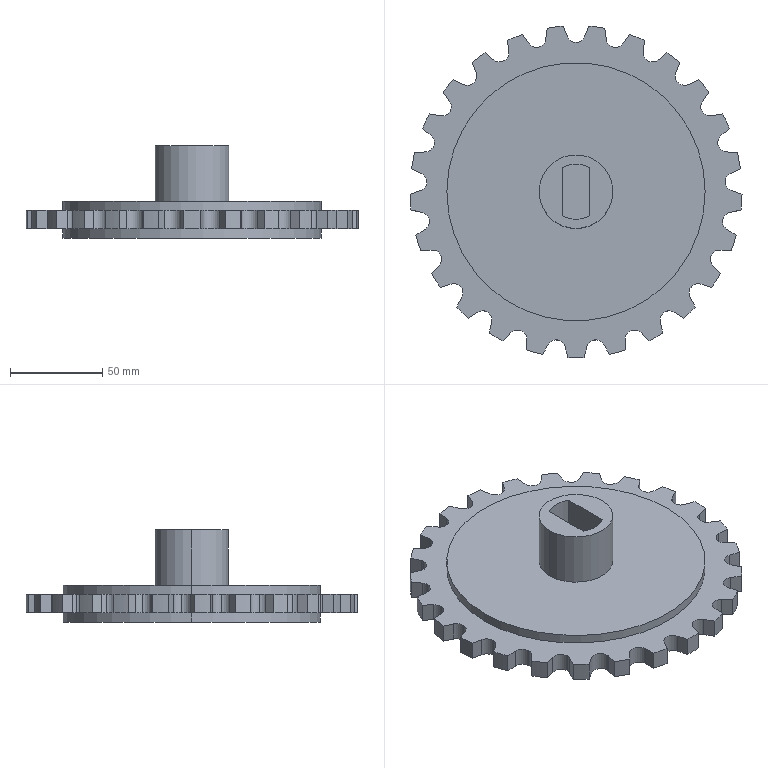Part | SolidWorks | 1 solid | 125 faces | box 179.981 x 179.731 x 50 mm | volume 415384 mm3 | cylinder 67 | plane 58 | commonest cylinder face diameters 10 x34 180 x25 140 x4 30 x2 40 x2